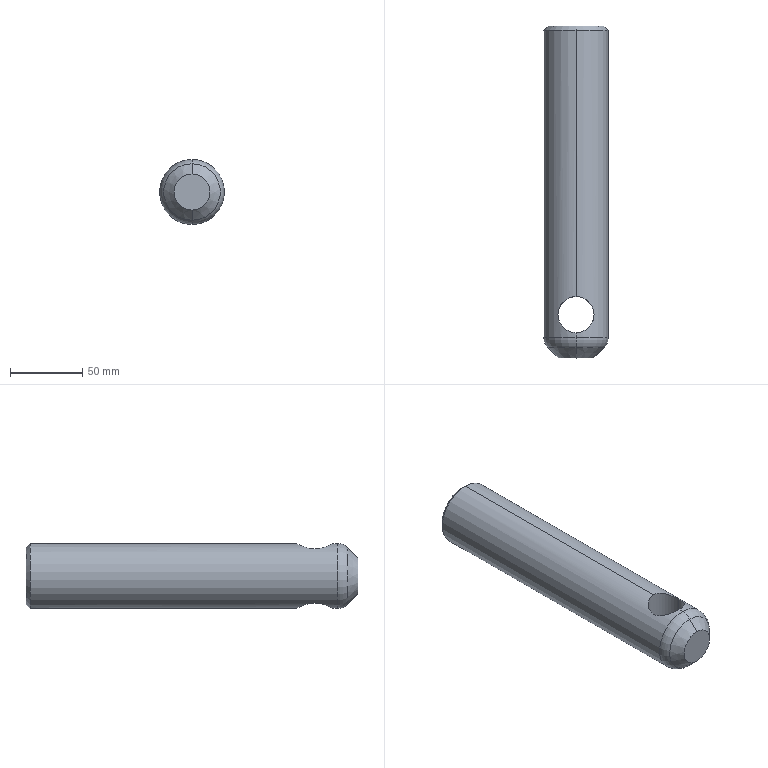Part | SolidWorks | features ICE 3, Chamfer 2, Extrusion 1, Fillet 1 | 1 solid | 15 faces | box 45 x 230 x 45 mm | volume 210439 mm3 | cylinder 6 | cone 4 | plane 3 | torus 2 | commonest cylinder face diameters 25 x2 30 x2 45 x2
STEP:
#1=CARTESIAN_POINT('',(0.,14.142,22.5));
#2=VERTEX_POINT('',#1);
#3=CARTESIAN_POINT('',(0.,14.142,-22.5));
#4=VERTEX_POINT('',#3);
#5=CARTESIAN_POINT('',(0.,14.142,0.));
#6=DIRECTION('',(0.,1.,0.));
#7=DIRECTION('',(0.,0.,-1.));
#8=AXIS2_PLACEMENT_3D('',#5,#6,#7);
#9=CIRCLE('',#8,22.5);
#10=EDGE_CURVE('',#2,#4,#9,.T.);
#11=ORIENTED_EDGE('',*,*,#10,.F.);
#12=CARTESIAN_POINT('',(0.,7.071,19.571));
#13=VERTEX_POINT('',#12);
#14=CARTESIAN_POINT('',(0.,14.142,12.5));
#15=DIRECTION('',(1.,0.,0.));
#16=DIRECTION('',(0.,0.,-1.));
#17=AXIS2_PLACEMENT_3D('',#14,#15,#16);
#18=CIRCLE('',#17,10.);
#19=EDGE_CURVE('',#2,#13,#18,.T.);
#20=ORIENTED_EDGE('',*,*,#19,.T.);
#21=CARTESIAN_POINT('',(0.,7.071,-19.571));
#22=VERTEX_POINT('',#21);
#23=CARTESIAN_POINT('',(0.,7.071,0.));
#24=DIRECTION('',(0.,-1.,0.));
#25=DIRECTION('',(0.,0.,1.));
#26=AXIS2_PLACEMENT_3D('',#23,#24,#25);
#27=CIRCLE('',#26,19.571);
#28=EDGE_CURVE('',#22,#13,#27,.T.);
#29=ORIENTED_EDGE('',*,*,#28,.F.);
#30=CARTESIAN_POINT('',(0.,14.142,-12.5));
#31=DIRECTION('',(-1.,0.,0.));
#32=DIRECTION('',(0.,0.,1.));
#33=AXIS2_PLACEMENT_3D('',#30,#31,#32);
#34=CIRCLE('',#33,10.);
#35=EDGE_CURVE('',#4,#22,#34,.T.);
#36=ORIENTED_EDGE('',*,*,#35,.F.);
#37=EDGE_LOOP('',(#11,#20,#29,#36));
#38=FACE_OUTER_BOUND('',#37,.T.);
#39=CARTESIAN_POINT('',(0.,14.142,0.));
#40=DIRECTION('',(0.,-1.,0.));
#41=DIRECTION('',(0.,0.,-1.));
#42=AXIS2_PLACEMENT_3D('',#39,#40,#41);
#43=TOROIDAL_SURFACE('',#42,12.5,10.);
#44=ADVANCED_FACE('',(#38),#43,.T.);
#45=CARTESIAN_POINT('',(0.,230.,19.5));
#46=VERTEX_POINT('',#45);
#47=CARTESIAN_POINT('',(0.,230.,-19.5));
#48=VERTEX_POINT('',#47);
#49=CARTESIAN_POINT('',(0.,230.,0.));
#50=DIRECTION('',(0.,1.,0.));
#51=DIRECTION('',(0.,0.,1.));
#52=AXIS2_PLACEMENT_3D('',#49,#50,#51);
#53=CIRCLE('',#52,19.5);
#54=EDGE_CURVE('',#46,#48,#53,.T.);
#55=ORIENTED_EDGE('',*,*,#54,.F.);
#56=CARTESIAN_POINT('',(0.,227.,22.5));
#57=VERTEX_POINT('',#56);
#58=CARTESIAN_POINT('',(0.,230.,19.5));
#59=DIRECTION('',(0.,-0.7071,0.7071));
#60=VECTOR('',#59,1000.);
#61=LINE('',#58,#60);
#62=EDGE_CURVE('',#46,#57,#61,.T.);
#63=ORIENTED_EDGE('',*,*,#62,.T.);
#64=CARTESIAN_POINT('',(0.,227.,-22.5));
#65=VERTEX_POINT('',#64);
#66=CARTESIAN_POINT('',(0.,227.,0.));
#67=DIRECTION('',(0.,-1.,0.));
#68=DIRECTION('',(0.,0.,1.));
#69=AXIS2_PLACEMENT_3D('',#66,#67,#68);
#70=CIRCLE('',#69,22.5);
#71=EDGE_CURVE('',#65,#57,#70,.T.);
#72=ORIENTED_EDGE('',*,*,#71,.F.);
#73=CARTESIAN_POINT('',(0.,230.,-19.5));
#74=DIRECTION('',(0.,-0.7071,-0.7071));
#75=VECTOR('',#74,1000.);
#76=LINE('',#73,#75);
#77=EDGE_CURVE('',#48,#65,#76,.T.);
#78=ORIENTED_EDGE('',*,*,#77,.F.);
#79=EDGE_LOOP('',(#55,#63,#72,#78));
#80=FACE_OUTER_BOUND('',#79,.T.);
#81=CARTESIAN_POINT('',(0.,230.,0.));
#82=DIRECTION('',(0.,-1.,0.));
#83=DIRECTION('',(0.,0.,-1.));
#84=AXIS2_PLACEMENT_3D('',#81,#82,#83);
#85=CONICAL_SURFACE('',#84,19.5,0.7854);
#86=ADVANCED_FACE('',(#80),#85,.T.);
#87=CARTESIAN_POINT('',(0.,0.,-12.5));
#88=VERTEX_POINT('',#87);
#89=CARTESIAN_POINT('',(0.,0.,12.5));
#90=VERTEX_POINT('',#89);
#91=CARTESIAN_POINT('',(0.,0.,0.));
#92=DIRECTION('',(0.,-1.,0.));
#93=DIRECTION('',(0.,0.,1.));
#94=AXIS2_PLACEMENT_3D('',#91,#92,#93);
#95=CIRCLE('',#94,12.5);
#96=EDGE_CURVE('',#88,#90,#95,.T.);
#97=ORIENTED_EDGE('',*,*,#96,.F.);
#98=CARTESIAN_POINT('',(0.,10.,-22.5));
#99=DIRECTION('',(0.,0.7071,-0.7071));
#100=VECTOR('',#99,1000.);
#101=LINE('',#98,#100);
#102=EDGE_CURVE('',#88,#22,#101,.T.);
#103=ORIENTED_EDGE('',*,*,#102,.T.);
#104=ORIENTED_EDGE('',*,*,#28,.T.);
#105=CARTESIAN_POINT('',(0.,10.,22.5));
#106=DIRECTION('',(0.,0.7071,0.7071));
#107=VECTOR('',#106,1000.);
#108=LINE('',#105,#107);
#109=EDGE_CURVE('',#90,#13,#108,.T.);
#110=ORIENTED_EDGE('',*,*,#109,.F.);
#111=EDGE_LOOP('',(#97,#103,#104,#110));
#112=FACE_OUTER_BOUND('',#111,.T.);
#113=CARTESIAN_POINT('',(0.,10.,0.));
#114=DIRECTION('',(0.,1.,0.));
#115=DIRECTION('',(0.,0.,1.));
#116=AXIS2_PLACEMENT_3D('',#113,#114,#115);
#117=CONICAL_SURFACE('',#116,22.5,0.7854);
#118=ADVANCED_FACE('',(#112),#117,.T.);
#119=CARTESIAN_POINT('',(0.,50.,-15.));
#120=VERTEX_POINT('',#119);
#121=CARTESIAN_POINT('',(0.,50.,15.));
#122=VERTEX_POINT('',#121);
#123=CARTESIAN_POINT('',(0.,50.,0.));
#124=DIRECTION('',(0.,1.,0.));
#125=DIRECTION('',(0.,0.,1.));
#126=AXIS2_PLACEMENT_3D('',#123,#124,#125);
#127=CIRCLE('',#126,15.);
#128=EDGE_CURVE('',#120,#122,#127,.T.);
#129=ORIENTED_EDGE('',*,*,#128,.F.);
#130=CARTESIAN_POINT('',(0.,230.,-15.));
#131=VERTEX_POINT('',#130);
#132=CARTESIAN_POINT('',(0.,50.,-15.));
#133=DIRECTION('',(0.,1.,0.));
#134=VECTOR('',#133,1000.);
#135=LINE('',#132,#134);
#136=EDGE_CURVE('',#120,#131,#135,.T.);
#137=ORIENTED_EDGE('',*,*,#136,.T.);
#138=CARTESIAN_POINT('',(0.,230.,15.));
#139=VERTEX_POINT('',#138);
#140=CARTESIAN_POINT('',(0.,230.,0.));
#141=DIRECTION('',(0.,-1.,0.));
#142=DIRECTION('',(0.,0.,1.));
#143=AXIS2_PLACEMENT_3D('',#140,#141,#142);
#144=CIRCLE('',#143,15.);
#145=EDGE_CURVE('',#139,#131,#144,.T.);
#146=ORIENTED_EDGE('',*,*,#145,.F.);
#147=CARTESIAN_POINT('',(0.,50.,15.));
#148=DIRECTION('',(0.,1.,0.));
#149=VECTOR('',#148,1000.);
#150=LINE('',#147,#149);
#151=EDGE_CURVE('',#122,#139,#150,.T.);
#152=ORIENTED_EDGE('',*,*,#151,.F.);
#153=EDGE_LOOP('',(#129,#137,#146,#152));
#154=FACE_OUTER_BOUND('',#153,.T.);
#155=CARTESIAN_POINT('',(0.,50.,0.));
#156=DIRECTION('',(0.,1.,0.));
#157=DIRECTION('',(0.,0.,1.));
#158=AXIS2_PLACEMENT_3D('',#155,#156,#157);
#159=CYLINDRICAL_SURFACE('',#158,15.);
#160=ADVANCED_FACE('',(#154),#159,.F.);
#161=CARTESIAN_POINT('',(0.,17.5,22.5));
#162=VERTEX_POINT('',#161);
#163=CARTESIAN_POINT('',(12.5,30.,18.708));
#164=VERTEX_POINT('',#163);
#165=CARTESIAN_POINT('',(0.,17.5,22.5));
#166=CARTESIAN_POINT('',(0.4191,17.5,22.5));
#167=CARTESIAN_POINT('',(0.8433,17.521,22.488));
#168=CARTESIAN_POINT('',(1.676,17.606,22.441));
#169=CARTESIAN_POINT('',(2.087,17.669,22.407));
#170=CARTESIAN_POINT('',(2.899,17.834,22.316));
#171=CARTESIAN_POINT('',(3.3,17.936,22.26));
#172=CARTESIAN_POINT('',(4.092,18.181,22.128));
#173=CARTESIAN_POINT('',(4.484,18.325,22.052));
#174=CARTESIAN_POINT('',(5.62,18.804,21.801));
#175=CARTESIAN_POINT('',(6.332,19.192,21.602));
#176=CARTESIAN_POINT('',(7.339,19.873,21.272));
#177=CARTESIAN_POINT('',(7.665,20.117,21.157));
#178=CARTESIAN_POINT('',(8.285,20.631,20.922));
#179=CARTESIAN_POINT('',(8.58,20.901,20.802));
#180=CARTESIAN_POINT('',(9.143,21.467,20.561));
#181=CARTESIAN_POINT('',(9.411,21.763,20.439));
#182=CARTESIAN_POINT('',(9.919,22.382,20.198));
#183=CARTESIAN_POINT('',(10.16,22.707,20.077));
#184=CARTESIAN_POINT('',(10.835,23.714,19.726));
#185=CARTESIAN_POINT('',(11.216,24.422,19.509));
#186=CARTESIAN_POINT('',(11.685,25.542,19.229));
#187=CARTESIAN_POINT('',(11.825,25.926,19.143));
#188=CARTESIAN_POINT('',(12.067,26.714,18.991));
#189=CARTESIAN_POINT('',(12.171,27.121,18.924));
#190=CARTESIAN_POINT('',(12.417,28.342,18.764));
#191=CARTESIAN_POINT('',(12.5,29.166,18.708));
#192=CARTESIAN_POINT('',(12.5,30.,18.708));
#193=B_SPLINE_CURVE_WITH_KNOTS('',3,(#165,#166,#167,#168,#169,#170,#171,#172,#173,#174,#175,#176,#177,#178,#179,#180,#181,#182,#183,#184,#185,#186,#187,#188,#189,#190,#191,#192),.UNSPECIFIED.,.F.,.F.,(4,2,2,2,2,2,2,2,2,2,2,2,2,4),(0.01998,0.02123,0.02247,0.02372,0.02497,0.02746,0.02871,0.02996,0.03121,0.03245,0.03495,0.0362,0.03745,0.03994),.UNSPECIFIED.);
#194=EDGE_CURVE('',#162,#164,#193,.T.);
#195=ORIENTED_EDGE('',*,*,#194,.T.);
#196=CARTESIAN_POINT('',(12.5,30.,-18.708));
#197=VERTEX_POINT('',#196);
#198=CARTESIAN_POINT('',(12.5,30.,210.));
#199=DIRECTION('',(0.,0.,-1.));
#200=VECTOR('',#199,1000.);
#201=LINE('',#198,#200);
#202=EDGE_CURVE('',#164,#197,#201,.T.);
#203=ORIENTED_EDGE('',*,*,#202,.T.);
#204=CARTESIAN_POINT('',(0.,17.5,-22.5));
#205=VERTEX_POINT('',#204);
#206=CARTESIAN_POINT('',(12.5,30.,-18.708));
#207=CARTESIAN_POINT('',(12.5,29.155,-18.708));
#208=CARTESIAN_POINT('',(12.415,28.326,-18.766));
#209=CARTESIAN_POINT('',(12.168,27.108,-18.926));
#210=CARTESIAN_POINT('',(12.065,26.705,-18.992));
#211=CARTESIAN_POINT('',(11.82,25.913,-19.146));
#212=CARTESIAN_POINT('',(11.679,25.527,-19.232));
#213=CARTESIAN_POINT('',(11.364,24.777,-19.42));
#214=CARTESIAN_POINT('',(11.188,24.411,-19.522));
#215=CARTESIAN_POINT('',(10.803,23.699,-19.738));
#216=CARTESIAN_POINT('',(10.593,23.351,-19.852));
#217=CARTESIAN_POINT('',(9.916,22.346,-20.204));
#218=CARTESIAN_POINT('',(9.408,21.73,-20.448));
#219=CARTESIAN_POINT('',(8.56,20.882,-20.81));
#220=CARTESIAN_POINT('',(8.263,20.612,-20.93));
#221=CARTESIAN_POINT('',(7.638,20.097,-21.166));
#222=CARTESIAN_POINT('',(7.314,19.855,-21.281));
#223=CARTESIAN_POINT('',(6.312,19.181,-21.608));
#224=CARTESIAN_POINT('',(5.603,18.796,-21.805));
#225=CARTESIAN_POINT('',(4.471,18.32,-22.055));
#226=CARTESIAN_POINT('',(4.08,18.177,-22.131));
#227=CARTESIAN_POINT('',(3.286,17.932,-22.262));
#228=CARTESIAN_POINT('',(2.885,17.83,-22.318));
#229=CARTESIAN_POINT('',(1.67,17.584,-22.453));
#230=CARTESIAN_POINT('',(0.8436,17.5,-22.5));
#231=CARTESIAN_POINT('',(0.,17.5,-22.5));
#232=B_SPLINE_CURVE_WITH_KNOTS('',3,(#206,#207,#208,#209,#210,#211,#212,#213,#214,#215,#216,#217,#218,#219,#220,#221,#222,#223,#224,#225,#226,#227,#228,#229,#230,#231),.UNSPECIFIED.,.F.,.F.,(4,2,2,2,2,2,2,2,2,2,2,2,4),(0.01997,0.02247,0.02371,0.02496,0.02621,0.02746,0.02995,0.0312,0.03245,0.03494,0.03619,0.03744,0.03994),.UNSPECIFIED.);
#233=EDGE_CURVE('',#197,#205,#232,.T.);
#234=ORIENTED_EDGE('',*,*,#233,.T.);
#235=CARTESIAN_POINT('',(-12.5,30.,-18.708));
#236=VERTEX_POINT('',#235);
#237=CARTESIAN_POINT('',(0.,17.5,-22.5));
#238=CARTESIAN_POINT('',(-0.4212,17.5,-22.5));
#239=CARTESIAN_POINT('',(-0.8421,17.521,-22.488));
#240=CARTESIAN_POINT('',(-1.671,17.605,-22.442));
#241=CARTESIAN_POINT('',(-2.082,17.668,-22.407));
#242=CARTESIAN_POINT('',(-2.893,17.832,-22.317));
#243=CARTESIAN_POINT('',(-3.295,17.935,-22.261));
#244=CARTESIAN_POINT('',(-4.09,18.181,-22.129));
#245=CARTESIAN_POINT('',(-4.479,18.323,-22.053));
#246=CARTESIAN_POINT('',(-5.611,18.8,-21.803));
#247=CARTESIAN_POINT('',(-6.324,19.187,-21.605));
#248=CARTESIAN_POINT('',(-7.334,19.87,-21.274));
#249=CARTESIAN_POINT('',(-7.658,20.113,-21.159));
#250=CARTESIAN_POINT('',(-8.277,20.624,-20.925));
#251=CARTESIAN_POINT('',(-8.572,20.893,-20.806));
#252=CARTESIAN_POINT('',(-9.135,21.458,-20.564));
#253=CARTESIAN_POINT('',(-9.403,21.754,-20.443));
#254=CARTESIAN_POINT('',(-9.913,22.375,-20.2));
#255=CARTESIAN_POINT('',(-10.155,22.7,-20.08));
#256=CARTESIAN_POINT('',(-10.827,23.701,-19.73));
#257=CARTESIAN_POINT('',(-11.208,24.407,-19.513));
#258=CARTESIAN_POINT('',(-11.68,25.528,-19.232));
#259=CARTESIAN_POINT('',(-11.82,25.913,-19.146));
#260=CARTESIAN_POINT('',(-12.065,26.705,-18.992));
#261=CARTESIAN_POINT('',(-12.168,27.108,-18.926));
#262=CARTESIAN_POINT('',(-12.415,28.325,-18.766));
#263=CARTESIAN_POINT('',(-12.5,29.155,-18.708));
#264=CARTESIAN_POINT('',(-12.5,30.,-18.708));
#265=B_SPLINE_CURVE_WITH_KNOTS('',3,(#237,#238,#239,#240,#241,#242,#243,#244,#245,#246,#247,#248,#249,#250,#251,#252,#253,#254,#255,#256,#257,#258,#259,#260,#261,#262,#263,#264),.UNSPECIFIED.,.F.,.F.,(4,2,2,2,2,2,2,2,2,2,2,2,2,4),(0.03994,0.04118,0.04243,0.04367,0.04492,0.04741,0.04866,0.0499,0.05115,0.0524,0.05489,0.05614,0.05738,0.05987),.UNSPECIFIED.);
#266=EDGE_CURVE('',#205,#236,#265,.T.);
#267=ORIENTED_EDGE('',*,*,#266,.T.);
#268=CARTESIAN_POINT('',(-12.5,30.,18.708));
#269=VERTEX_POINT('',#268);
#270=CARTESIAN_POINT('',(-12.5,30.,210.));
#271=DIRECTION('',(0.,0.,-1.));
#272=VECTOR('',#271,1000.);
#273=LINE('',#270,#272);
#274=EDGE_CURVE('',#269,#236,#273,.T.);
#275=ORIENTED_EDGE('',*,*,#274,.F.);
#276=CARTESIAN_POINT('',(-12.5,30.,18.708));
#277=CARTESIAN_POINT('',(-12.5,29.154,18.708));
#278=CARTESIAN_POINT('',(-12.415,28.326,18.766));
#279=CARTESIAN_POINT('',(-12.168,27.11,18.926));
#280=CARTESIAN_POINT('',(-12.066,26.71,18.991));
#281=CARTESIAN_POINT('',(-11.821,25.916,19.145));
#282=CARTESIAN_POINT('',(-11.68,25.529,19.232));
#283=CARTESIAN_POINT('',(-11.206,24.403,19.514));
#284=CARTESIAN_POINT('',(-10.822,23.693,19.733));
#285=CARTESIAN_POINT('',(-9.918,22.349,20.202));
#286=CARTESIAN_POINT('',(-9.408,21.731,20.448));
#287=CARTESIAN_POINT('',(-8.561,20.883,20.81));
#288=CARTESIAN_POINT('',(-8.265,20.614,20.93));
#289=CARTESIAN_POINT('',(-7.643,20.101,21.165));
#290=CARTESIAN_POINT('',(-7.316,19.857,21.28));
#291=CARTESIAN_POINT('',(-6.31,19.18,21.608));
#292=CARTESIAN_POINT('',(-5.6,18.795,21.805));
#293=CARTESIAN_POINT('',(-4.472,18.32,22.054));
#294=CARTESIAN_POINT('',(-4.085,18.179,22.13));
#295=CARTESIAN_POINT('',(-3.289,17.933,22.262));
#296=CARTESIAN_POINT('',(-2.884,17.83,22.318));
#297=CARTESIAN_POINT('',(-1.665,17.584,22.453));
#298=CARTESIAN_POINT('',(-0.839,17.5,22.5));
#299=CARTESIAN_POINT('',(0.,17.5,22.5));
#300=B_SPLINE_CURVE_WITH_KNOTS('',3,(#276,#277,#278,#279,#280,#281,#282,#283,#284,#285,#286,#287,#288,#289,#290,#291,#292,#293,#294,#295,#296,#297,#298,#299),.UNSPECIFIED.,.F.,.F.,(4,2,2,2,2,2,2,2,2,2,2,4),(0.,0.002497,0.003746,0.004995,0.007492,0.00999,0.01124,0.01249,0.01498,0.01623,0.01748,0.01998),.UNSPECIFIED.);
#301=EDGE_CURVE('',#269,#162,#300,.T.);
#302=ORIENTED_EDGE('',*,*,#301,.T.);
#303=EDGE_LOOP('',(#195,#203,#234,#267,#275,#302));
#304=FACE_OUTER_BOUND('',#303,.T.);
#305=CARTESIAN_POINT('',(0.,30.,210.));
#306=DIRECTION('',(0.,0.,-1.));
#307=DIRECTION('',(-1.,0.,0.));
#308=AXIS2_PLACEMENT_3D('',#305,#306,#307);
#309=CYLINDRICAL_SURFACE('',#308,12.5);
#310=ADVANCED_FACE('',(#304),#309,.F.);
#311=ORIENTED_EDGE('',*,*,#71,.T.);
#312=CARTESIAN_POINT('',(0.,42.5,22.5));
#313=VERTEX_POINT('',#312);
#314=CARTESIAN_POINT('',(0.,250.,22.5));
#315=DIRECTION('',(0.,-1.,0.));
#316=VECTOR('',#315,1000.);
#317=LINE('',#314,#316);
#318=EDGE_CURVE('',#57,#313,#317,.T.);
#319=ORIENTED_EDGE('',*,*,#318,.T.);
#320=CARTESIAN_POINT('',(12.5,30.,18.708));
#321=CARTESIAN_POINT('',(12.5,30.416,18.708));
#322=CARTESIAN_POINT('',(12.479,30.838,18.722));
#323=CARTESIAN_POINT('',(12.394,31.675,18.778));
#324=CARTESIAN_POINT('',(12.332,32.086,18.82));
#325=CARTESIAN_POINT('',(12.167,32.897,18.927));
#326=CARTESIAN_POINT('',(12.065,33.297,18.993));
#327=CARTESIAN_POINT('',(11.821,34.083,19.145));
#328=CARTESIAN_POINT('',(11.68,34.472,19.232));
#329=CARTESIAN_POINT('',(11.203,35.605,19.516));
#330=CARTESIAN_POINT('',(10.818,36.314,19.735));
#331=CARTESIAN_POINT('',(10.144,37.315,20.085));
#332=CARTESIAN_POINT('',(9.901,37.64,20.206));
#333=CARTESIAN_POINT('',(9.39,38.261,20.449));
#334=CARTESIAN_POINT('',(9.121,38.557,20.571));
#335=CARTESIAN_POINT('',(8.275,39.403,20.932));
#336=CARTESIAN_POINT('',(7.658,39.913,21.169));
#337=CARTESIAN_POINT('',(6.308,40.822,21.609));
#338=CARTESIAN_POINT('',(5.593,41.208,21.807));
#339=CARTESIAN_POINT('',(4.469,41.681,22.055));
#340=CARTESIAN_POINT('',(4.084,41.821,22.13));
#341=CARTESIAN_POINT('',(3.296,42.065,22.261));
#342=CARTESIAN_POINT('',(2.89,42.169,22.317));
#343=CARTESIAN_POINT('',(1.66,42.417,22.454));
#344=CARTESIAN_POINT('',(0.8334,42.5,22.5));
#345=CARTESIAN_POINT('',(0.,42.5,22.5));
#346=B_SPLINE_CURVE_WITH_KNOTS('',3,(#320,#321,#322,#323,#324,#325,#326,#327,#328,#329,#330,#331,#332,#333,#334,#335,#336,#337,#338,#339,#340,#341,#342,#343,#344,#345),.UNSPECIFIED.,.F.,.F.,(4,2,2,2,2,2,2,2,2,2,2,2,4),(0.03994,0.04119,0.04243,0.04368,0.04492,0.04742,0.04866,0.04991,0.0524,0.05489,0.05614,0.05738,0.05987),.UNSPECIFIED.);
#347=EDGE_CURVE('',#164,#313,#346,.T.);
#348=ORIENTED_EDGE('',*,*,#347,.F.);
#349=ORIENTED_EDGE('',*,*,#194,.F.);
#350=CARTESIAN_POINT('',(0.,250.,22.5));
#351=DIRECTION('',(0.,-1.,0.));
#352=VECTOR('',#351,1000.);
#353=LINE('',#350,#352);
#354=EDGE_CURVE('',#162,#2,#353,.T.);
#355=ORIENTED_EDGE('',*,*,#354,.T.);
#356=ORIENTED_EDGE('',*,*,#10,.T.);
#357=CARTESIAN_POINT('',(0.,250.,-22.5));
#358=DIRECTION('',(0.,-1.,0.));
#359=VECTOR('',#358,1000.);
#360=LINE('',#357,#359);
#361=EDGE_CURVE('',#205,#4,#360,.T.);
#362=ORIENTED_EDGE('',*,*,#361,.F.);
#363=ORIENTED_EDGE('',*,*,#233,.F.);
#364=CARTESIAN_POINT('',(0.,42.5,-22.5));
#365=VERTEX_POINT('',#364);
#366=CARTESIAN_POINT('',(0.,42.5,-22.5));
#367=CARTESIAN_POINT('',(0.8452,42.5,-22.5));
#368=CARTESIAN_POINT('',(1.673,42.415,-22.453));
#369=CARTESIAN_POINT('',(2.891,42.168,-22.317));
#370=CARTESIAN_POINT('',(3.293,42.066,-22.261));
#371=CARTESIAN_POINT('',(4.088,41.82,-22.129));
#372=CARTESIAN_POINT('',(4.477,41.678,-22.053));
#373=CARTESIAN_POINT('',(5.609,41.201,-21.803));
#374=CARTESIAN_POINT('',(6.322,40.814,-21.605));
#375=CARTESIAN_POINT('',(7.331,40.132,-21.275));
#376=CARTESIAN_POINT('',(7.656,39.889,-21.16));
#377=CARTESIAN_POINT('',(8.275,39.377,-20.926));
#378=CARTESIAN_POINT('',(8.57,39.108,-20.806));
#379=CARTESIAN_POINT('',(9.134,38.543,-20.565));
#380=CARTESIAN_POINT('',(9.402,38.247,-20.443));
#381=CARTESIAN_POINT('',(9.912,37.627,-20.201));
#382=CARTESIAN_POINT('',(10.154,37.301,-20.08));
#383=CARTESIAN_POINT('',(10.827,36.299,-19.73));
#384=CARTESIAN_POINT('',(11.208,35.594,-19.513));
#385=CARTESIAN_POINT('',(11.68,34.472,-19.232));
#386=CARTESIAN_POINT('',(11.82,34.088,-19.146));
#387=CARTESIAN_POINT('',(12.065,33.296,-18.993));
#388=CARTESIAN_POINT('',(12.168,32.892,-18.926));
#389=CARTESIAN_POINT('',(12.415,31.674,-18.766));
#390=CARTESIAN_POINT('',(12.5,30.846,-18.708));
#391=CARTESIAN_POINT('',(12.5,30.,-18.708));
#392=B_SPLINE_CURVE_WITH_KNOTS('',3,(#366,#367,#368,#369,#370,#371,#372,#373,#374,#375,#376,#377,#378,#379,#380,#381,#382,#383,#384,#385,#386,#387,#388,#389,#390,#391),.UNSPECIFIED.,.F.,.F.,(4,2,2,2,2,2,2,2,2,2,2,2,4),(0.,0.002496,0.003745,0.004993,0.007489,0.008737,0.009986,0.01123,0.01248,0.01498,0.01623,0.01747,0.01997),.UNSPECIFIED.);
#393=EDGE_CURVE('',#365,#197,#392,.T.);
#394=ORIENTED_EDGE('',*,*,#393,.F.);
#395=CARTESIAN_POINT('',(0.,250.,-22.5));
#396=DIRECTION('',(0.,-1.,0.));
#397=VECTOR('',#396,1000.);
#398=LINE('',#395,#397);
#399=EDGE_CURVE('',#65,#365,#398,.T.);
#400=ORIENTED_EDGE('',*,*,#399,.F.);
#401=EDGE_LOOP('',(#311,#319,#348,#349,#355,#356,#362,#363,#394,#400));
#402=FACE_OUTER_BOUND('',#401,.T.);
#403=CARTESIAN_POINT('',(0.,250.,0.));
#404=DIRECTION('',(0.,-1.,0.));
#405=DIRECTION('',(0.,0.,-1.));
#406=AXIS2_PLACEMENT_3D('',#403,#404,#405);
#407=CYLINDRICAL_SURFACE('',#406,22.5);
#408=ADVANCED_FACE('',(#402),#407,.T.);
#409=ORIENTED_EDGE('',*,*,#318,.F.);
#410=CARTESIAN_POINT('',(0.,227.,0.));
#411=DIRECTION('',(0.,-1.,0.));
#412=DIRECTION('',(0.,0.,1.));
#413=AXIS2_PLACEMENT_3D('',#410,#411,#412);
#414=CIRCLE('',#413,22.5);
#415=EDGE_CURVE('',#57,#65,#414,.T.);
#416=ORIENTED_EDGE('',*,*,#415,.T.);
#417=ORIENTED_EDGE('',*,*,#399,.T.);
#418=CARTESIAN_POINT('',(-12.5,30.,-18.708));
#419=CARTESIAN_POINT('',(-12.5,30.845,-18.708));
#420=CARTESIAN_POINT('',(-12.415,31.673,-18.766));
#421=CARTESIAN_POINT('',(-12.168,32.891,-18.926));
#422=CARTESIAN_POINT('',(-12.065,33.294,-18.992));
#423=CARTESIAN_POINT('',(-11.821,34.086,-19.145));
#424=CARTESIAN_POINT('',(-11.68,34.471,-19.232));
#425=CARTESIAN_POINT('',(-11.364,35.222,-19.42));
#426=CARTESIAN_POINT('',(-11.189,35.587,-19.522));
#427=CARTESIAN_POINT('',(-10.804,36.299,-19.737));
#428=CARTESIAN_POINT('',(-10.594,36.648,-19.852));
#429=CARTESIAN_POINT('',(-9.917,37.652,-20.203));
#430=CARTESIAN_POINT('',(-9.409,38.268,-20.447));
#431=CARTESIAN_POINT('',(-8.279,39.399,-20.93));
#432=CARTESIAN_POINT('',(-7.65,39.918,-21.171));
#433=CARTESIAN_POINT('',(-6.315,40.817,-21.607));
#434=CARTESIAN_POINT('',(-5.606,41.202,-21.804));
#435=CARTESIAN_POINT('',(-4.474,41.679,-22.054));
#436=CARTESIAN_POINT('',(-4.082,41.822,-22.13));
#437=CARTESIAN_POINT('',(-3.289,42.067,-22.262));
#438=CARTESIAN_POINT('',(-2.888,42.169,-22.318));
#439=CARTESIAN_POINT('',(-1.673,42.415,-22.453));
#440=CARTESIAN_POINT('',(-0.8436,42.5,-22.5));
#441=CARTESIAN_POINT('',(0.,42.5,-22.5));
#442=B_SPLINE_CURVE_WITH_KNOTS('',3,(#418,#419,#420,#421,#422,#423,#424,#425,#426,#427,#428,#429,#430,#431,#432,#433,#434,#435,#436,#437,#438,#439,#440,#441),.UNSPECIFIED.,.F.,.F.,(4,2,2,2,2,2,2,2,2,2,2,4),(0.05987,0.06237,0.06361,0.06486,0.0661,0.06735,0.06984,0.07233,0.07482,0.07607,0.07732,0.07981),.UNSPECIFIED.);
#443=EDGE_CURVE('',#236,#365,#442,.T.);
#444=ORIENTED_EDGE('',*,*,#443,.F.);
#445=ORIENTED_EDGE('',*,*,#266,.F.);
#446=ORIENTED_EDGE('',*,*,#361,.T.);
#447=CARTESIAN_POINT('',(0.,14.142,0.));
#448=DIRECTION('',(0.,1.,0.));
#449=DIRECTION('',(0.,0.,-1.));
#450=AXIS2_PLACEMENT_3D('',#447,#448,#449);
#451=CIRCLE('',#450,22.5);
#452=EDGE_CURVE('',#4,#2,#451,.T.);
#453=ORIENTED_EDGE('',*,*,#452,.T.);
#454=ORIENTED_EDGE('',*,*,#354,.F.);
#455=ORIENTED_EDGE('',*,*,#301,.F.);
#456=CARTESIAN_POINT('',(0.,42.5,22.5));
#457=CARTESIAN_POINT('',(-0.416,42.5,22.5));
#458=CARTESIAN_POINT('',(-0.8337,42.479,22.488));
#459=CARTESIAN_POINT('',(-1.673,42.395,22.442));
#460=CARTESIAN_POINT('',(-2.085,42.332,22.407));
#461=CARTESIAN_POINT('',(-3.304,42.084,22.271));
#462=CARTESIAN_POINT('',(-4.092,41.84,22.138));
#463=CARTESIAN_POINT('',(-5.615,41.198,21.802));
#464=CARTESIAN_POINT('',(-6.327,40.81,21.603));
#465=CARTESIAN_POINT('',(-7.663,39.909,21.167));
#466=CARTESIAN_POINT('',(-8.29,39.389,20.926));
#467=CARTESIAN_POINT('',(-9.418,38.258,20.443));
#468=CARTESIAN_POINT('',(-9.924,37.643,20.199));
#469=CARTESIAN_POINT('',(-10.598,36.64,19.849));
#470=CARTESIAN_POINT('',(-10.809,36.292,19.735));
#471=CARTESIAN_POINT('',(-11.192,35.581,19.52));
#472=CARTESIAN_POINT('',(-11.366,35.217,19.419));
#473=CARTESIAN_POINT('',(-11.836,34.1,19.139));
#474=CARTESIAN_POINT('',(-12.08,33.321,18.983));
#475=CARTESIAN_POINT('',(-12.414,31.682,18.766));
#476=CARTESIAN_POINT('',(-12.5,30.843,18.708));
#477=CARTESIAN_POINT('',(-12.5,30.,18.708));
#478=B_SPLINE_CURVE_WITH_KNOTS('',3,(#456,#457,#458,#459,#460,#461,#462,#463,#464,#465,#466,#467,#468,#469,#470,#471,#472,#473,#474,#475,#476,#477),.UNSPECIFIED.,.F.,.F.,(4,2,2,2,2,2,2,2,2,2,4),(0.05987,0.06112,0.06236,0.06485,0.06734,0.06982,0.07231,0.07356,0.0748,0.07729,0.07978),.UNSPECIFIED.);
#479=EDGE_CURVE('',#313,#269,#478,.T.);
#480=ORIENTED_EDGE('',*,*,#479,.F.);
#481=EDGE_LOOP('',(#409,#416,#417,#444,#445,#446,#453,#454,#455,#480));
#482=FACE_OUTER_BOUND('',#481,.T.);
#483=CARTESIAN_POINT('',(0.,250.,0.));
#484=DIRECTION('',(0.,-1.,0.));
#485=DIRECTION('',(0.,0.,-1.));
#486=AXIS2_PLACEMENT_3D('',#483,#484,#485);
#487=CYLINDRICAL_SURFACE('',#486,22.5);
#488=ADVANCED_FACE('',(#482),#487,.T.);
#489=CARTESIAN_POINT('',(0.,0.,0.));
#490=DIRECTION('',(0.,-1.,0.));
#491=DIRECTION('',(0.,0.,1.));
#492=AXIS2_PLACEMENT_3D('',#489,#490,#491);
#493=CIRCLE('',#492,12.5);
#494=EDGE_CURVE('',#90,#88,#493,.T.);
#495=ORIENTED_EDGE('',*,*,#494,.T.);
#496=ORIENTED_EDGE('',*,*,#96,.T.);
#497=EDGE_LOOP('',(#495,#496));
#498=FACE_OUTER_BOUND('',#497,.T.);
#499=CARTESIAN_POINT('',(0.,0.,0.));
#500=DIRECTION('',(0.,1.,0.));
#501=DIRECTION('',(0.,0.,1.));
#502=AXIS2_PLACEMENT_3D('',#499,#500,#501);
#503=PLANE('',#502);
#504=ADVANCED_FACE('',(#498),#503,.F.);
#505=ORIENTED_EDGE('',*,*,#202,.F.);
#506=ORIENTED_EDGE('',*,*,#347,.T.);
#507=ORIENTED_EDGE('',*,*,#479,.T.);
#508=ORIENTED_EDGE('',*,*,#274,.T.);
#509=ORIENTED_EDGE('',*,*,#443,.T.);
#510=ORIENTED_EDGE('',*,*,#393,.T.);
#511=EDGE_LOOP('',(#505,#506,#507,#508,#509,#510));
#512=FACE_OUTER_BOUND('',#511,.T.);
#513=CARTESIAN_POINT('',(0.,30.,210.));
#514=DIRECTION('',(0.,0.,-1.));
#515=DIRECTION('',(-1.,0.,0.));
#516=AXIS2_PLACEMENT_3D('',#513,#514,#515);
#517=CYLINDRICAL_SURFACE('',#516,12.5);
#518=ADVANCED_FACE('',(#512),#517,.F.);
#519=CARTESIAN_POINT('',(0.,230.,0.));
#520=DIRECTION('',(0.,1.,0.));
#521=DIRECTION('',(0.,0.,1.));
#522=AXIS2_PLACEMENT_3D('',#519,#520,#521);
#523=CIRCLE('',#522,19.5);
#524=EDGE_CURVE('',#48,#46,#523,.T.);
#525=ORIENTED_EDGE('',*,*,#524,.T.);
#526=ORIENTED_EDGE('',*,*,#54,.T.);
#527=EDGE_LOOP('',(#525,#526));
#528=FACE_OUTER_BOUND('',#527,.T.);
#529=ORIENTED_EDGE('',*,*,#145,.T.);
#530=CARTESIAN_POINT('',(0.,230.,0.));
#531=DIRECTION('',(0.,-1.,0.));
#532=DIRECTION('',(0.,0.,1.));
#533=AXIS2_PLACEMENT_3D('',#530,#531,#532);
#534=CIRCLE('',#533,15.);
#535=EDGE_CURVE('',#131,#139,#534,.T.);
#536=ORIENTED_EDGE('',*,*,#535,.T.);
#537=EDGE_LOOP('',(#529,#536));
#538=FACE_BOUND('',#537,.T.);
#539=CARTESIAN_POINT('',(0.,230.,0.));
#540=DIRECTION('',(0.,1.,0.));
#541=DIRECTION('',(0.,0.,1.));
#542=AXIS2_PLACEMENT_3D('',#539,#540,#541);
#543=PLANE('',#542);
#544=ADVANCED_FACE('',(#528,#538),#543,.T.);
#545=CARTESIAN_POINT('',(0.,50.,0.));
#546=DIRECTION('',(0.,1.,0.));
#547=DIRECTION('',(0.,0.,1.));
#548=AXIS2_PLACEMENT_3D('',#545,#546,#547);
#549=CIRCLE('',#548,15.);
#550=EDGE_CURVE('',#122,#120,#549,.T.);
#551=ORIENTED_EDGE('',*,*,#550,.T.);
#552=ORIENTED_EDGE('',*,*,#128,.T.);
#553=EDGE_LOOP('',(#551,#552));
#554=FACE_OUTER_BOUND('',#553,.T.);
#555=CARTESIAN_POINT('',(0.,50.,0.));
#556=DIRECTION('',(0.,1.,0.));
#557=DIRECTION('',(0.,0.,1.));
#558=AXIS2_PLACEMENT_3D('',#555,#556,#557);
#559=PLANE('',#558);
#560=ADVANCED_FACE('',(#554),#559,.T.);
#561=ORIENTED_EDGE('',*,*,#136,.F.);
#562=ORIENTED_EDGE('',*,*,#550,.F.);
#563=ORIENTED_EDGE('',*,*,#151,.T.);
#564=ORIENTED_EDGE('',*,*,#535,.F.);
#565=EDGE_LOOP('',(#561,#562,#563,#564));
#566=FACE_OUTER_BOUND('',#565,.T.);
#567=CARTESIAN_POINT('',(0.,50.,0.));
#568=DIRECTION('',(0.,1.,0.));
#569=DIRECTION('',(0.,0.,1.));
#570=AXIS2_PLACEMENT_3D('',#567,#568,#569);
#571=CYLINDRICAL_SURFACE('',#570,15.);
#572=ADVANCED_FACE('',(#566),#571,.F.);
#573=ORIENTED_EDGE('',*,*,#102,.F.);
#574=ORIENTED_EDGE('',*,*,#494,.F.);
#575=ORIENTED_EDGE('',*,*,#109,.T.);
#576=CARTESIAN_POINT('',(0.,7.071,0.));
#577=DIRECTION('',(0.,-1.,0.));
#578=DIRECTION('',(0.,0.,1.));
#579=AXIS2_PLACEMENT_3D('',#576,#577,#578);
#580=CIRCLE('',#579,19.571);
#581=EDGE_CURVE('',#13,#22,#580,.T.);
#582=ORIENTED_EDGE('',*,*,#581,.T.);
#583=EDGE_LOOP('',(#573,#574,#575,#582));
#584=FACE_OUTER_BOUND('',#583,.T.);
#585=CARTESIAN_POINT('',(0.,10.,0.));
#586=DIRECTION('',(0.,1.,0.));
#587=DIRECTION('',(0.,0.,1.));
#588=AXIS2_PLACEMENT_3D('',#585,#586,#587);
#589=CONICAL_SURFACE('',#588,22.5,0.7854);
#590=ADVANCED_FACE('',(#584),#589,.T.);
#591=ORIENTED_EDGE('',*,*,#62,.F.);
#592=ORIENTED_EDGE('',*,*,#524,.F.);
#593=ORIENTED_EDGE('',*,*,#77,.T.);
#594=ORIENTED_EDGE('',*,*,#415,.F.);
#595=EDGE_LOOP('',(#591,#592,#593,#594));
#596=FACE_OUTER_BOUND('',#595,.T.);
#597=CARTESIAN_POINT('',(0.,230.,0.));
#598=DIRECTION('',(0.,-1.,0.));
#599=DIRECTION('',(0.,0.,-1.));
#600=AXIS2_PLACEMENT_3D('',#597,#598,#599);
#601=CONICAL_SURFACE('',#600,19.5,0.7854);
#602=ADVANCED_FACE('',(#596),#601,.T.);
#603=ORIENTED_EDGE('',*,*,#19,.F.);
#604=ORIENTED_EDGE('',*,*,#452,.F.);
#605=ORIENTED_EDGE('',*,*,#35,.T.);
#606=ORIENTED_EDGE('',*,*,#581,.F.);
#607=EDGE_LOOP('',(#603,#604,#605,#606));
#608=FACE_OUTER_BOUND('',#607,.T.);
#609=CARTESIAN_POINT('',(0.,14.142,0.));
#610=DIRECTION('',(0.,-1.,0.));
#611=DIRECTION('',(0.,0.,-1.));
#612=AXIS2_PLACEMENT_3D('',#609,#610,#611);
#613=TOROIDAL_SURFACE('',#612,12.5,10.);
#614=ADVANCED_FACE('',(#608),#613,.T.);
#615=CLOSED_SHELL('',(#44,#86,#118,#160,#310,#408,#488,#504,#518,#544,#560,#572,#590,#602,#614));
#616=MANIFOLD_SOLID_BREP('',#615);
#617=CARTESIAN_POINT('',(0.,0.,0.));
#618=DIRECTION('',(0.,0.,1.));
#619=DIRECTION('',(1.,0.,0.));
#620=AXIS2_PLACEMENT_3D('',#617,#618,#619);
#621=(LENGTH_UNIT()NAMED_UNIT(*)SI_UNIT(.MILLI.,.METRE.));
#622=UNCERTAINTY_MEASURE_WITH_UNIT(LENGTH_MEASURE(0.00001),#621,'','');
#623=(NAMED_UNIT(*)PLANE_ANGLE_UNIT()SI_UNIT($,.RADIAN.));
#624=(NAMED_UNIT(*)SI_UNIT($,.STERADIAN.)SOLID_ANGLE_UNIT());
#625=(GEOMETRIC_REPRESENTATION_CONTEXT(3)GLOBAL_UNCERTAINTY_ASSIGNED_CONTEXT((#622))GLOBAL_UNIT_ASSIGNED_CONTEXT((#621,#623,#624))REPRESENTATION_CONTEXT('',''));
#626=ADVANCED_BREP_SHAPE_REPRESENTATION('',(#616,#620),#625);